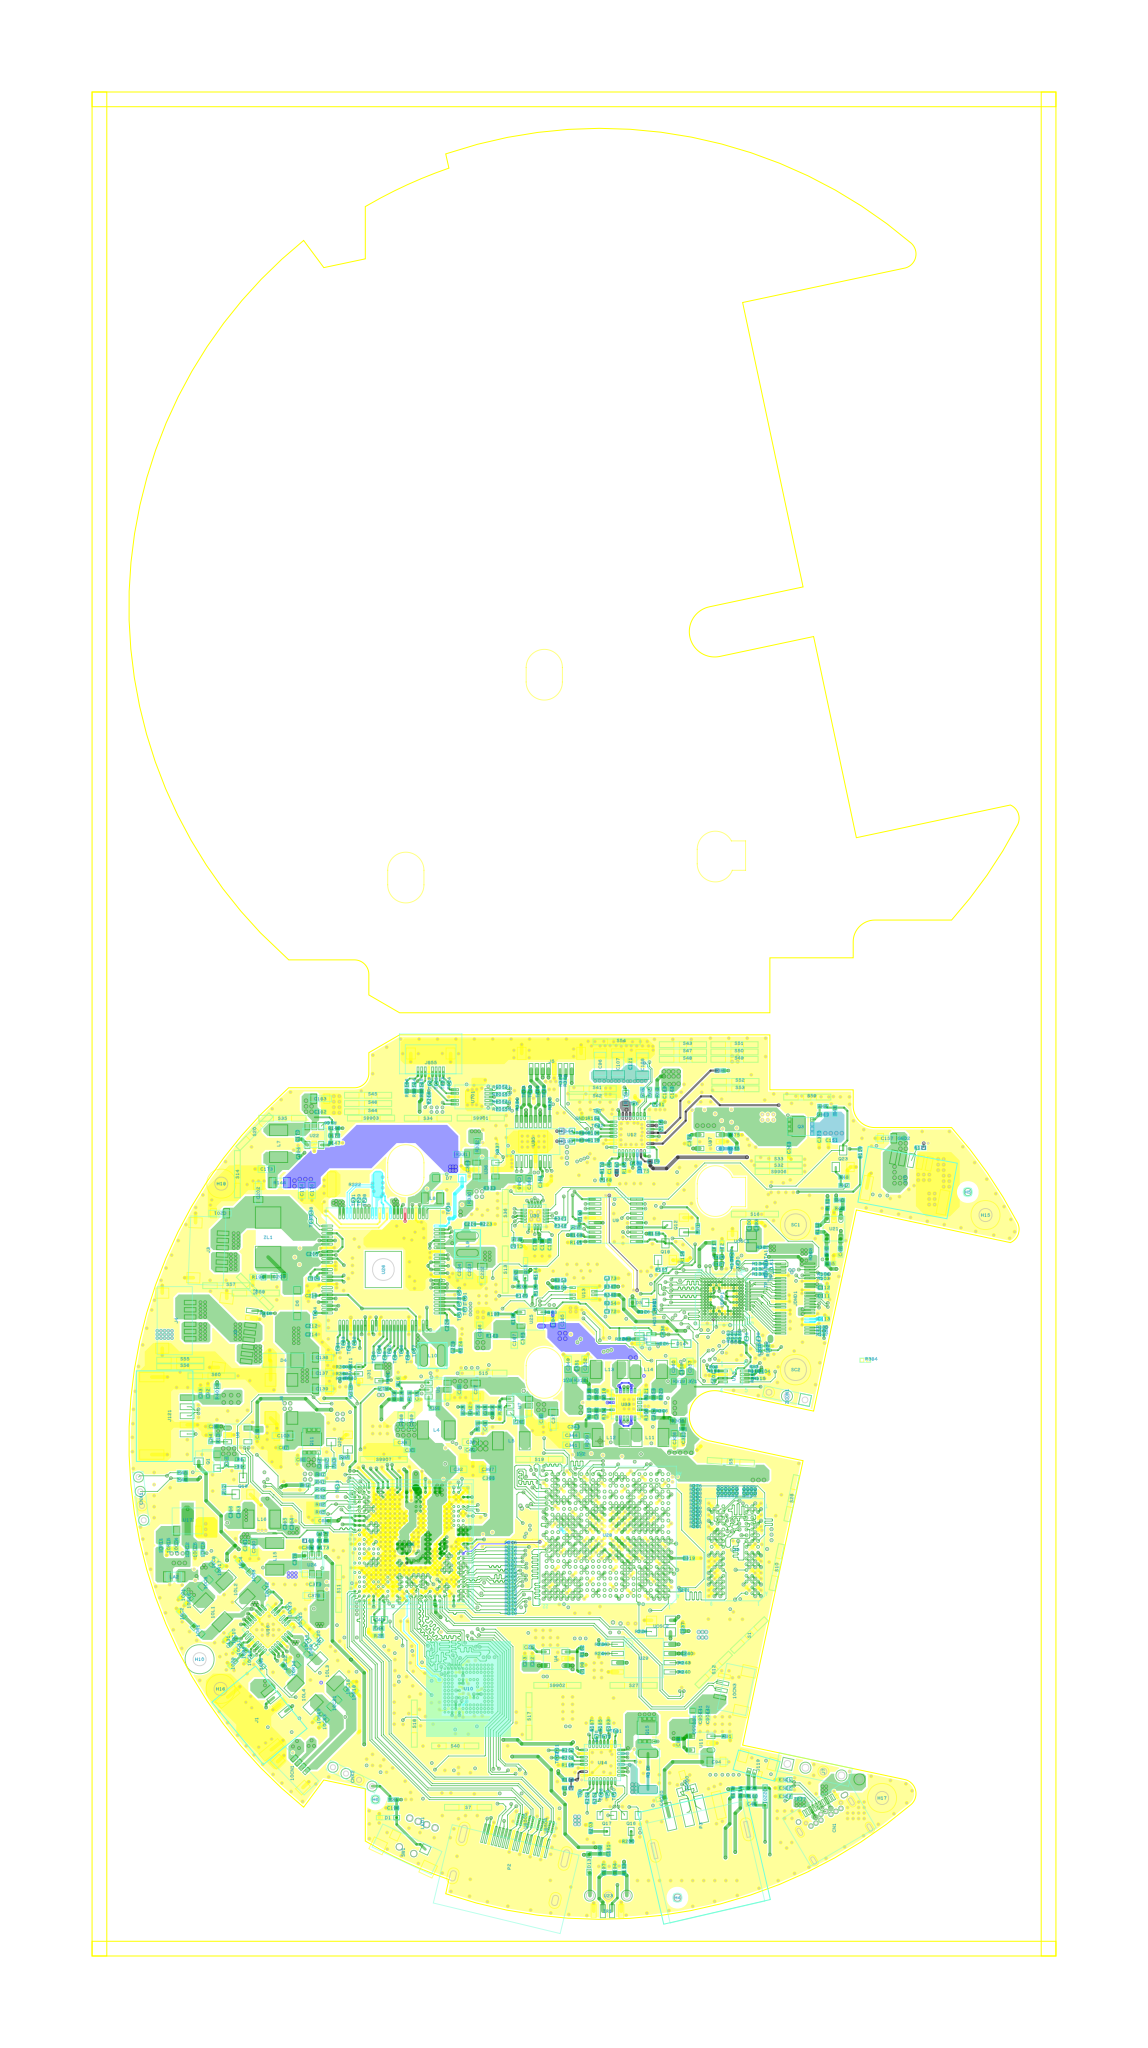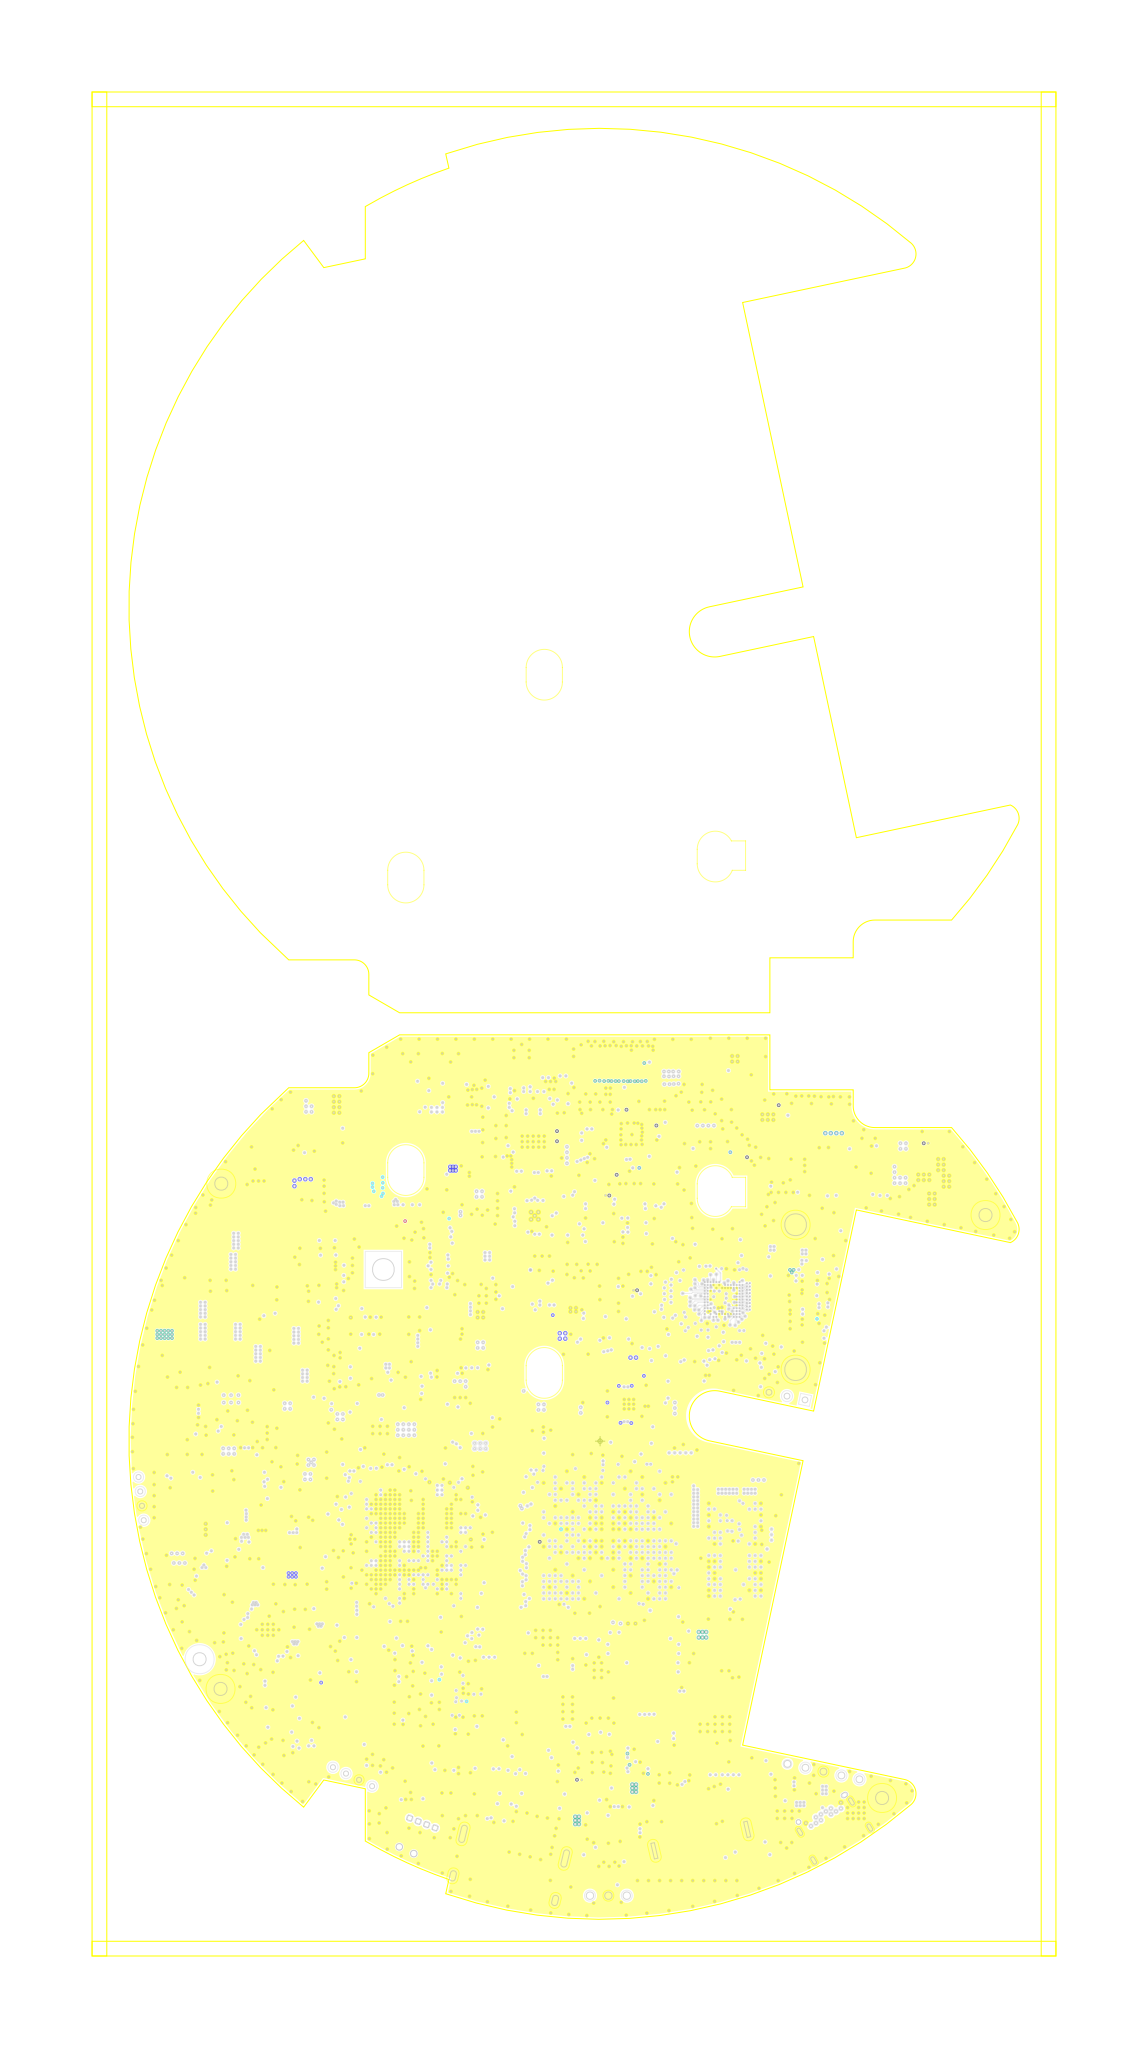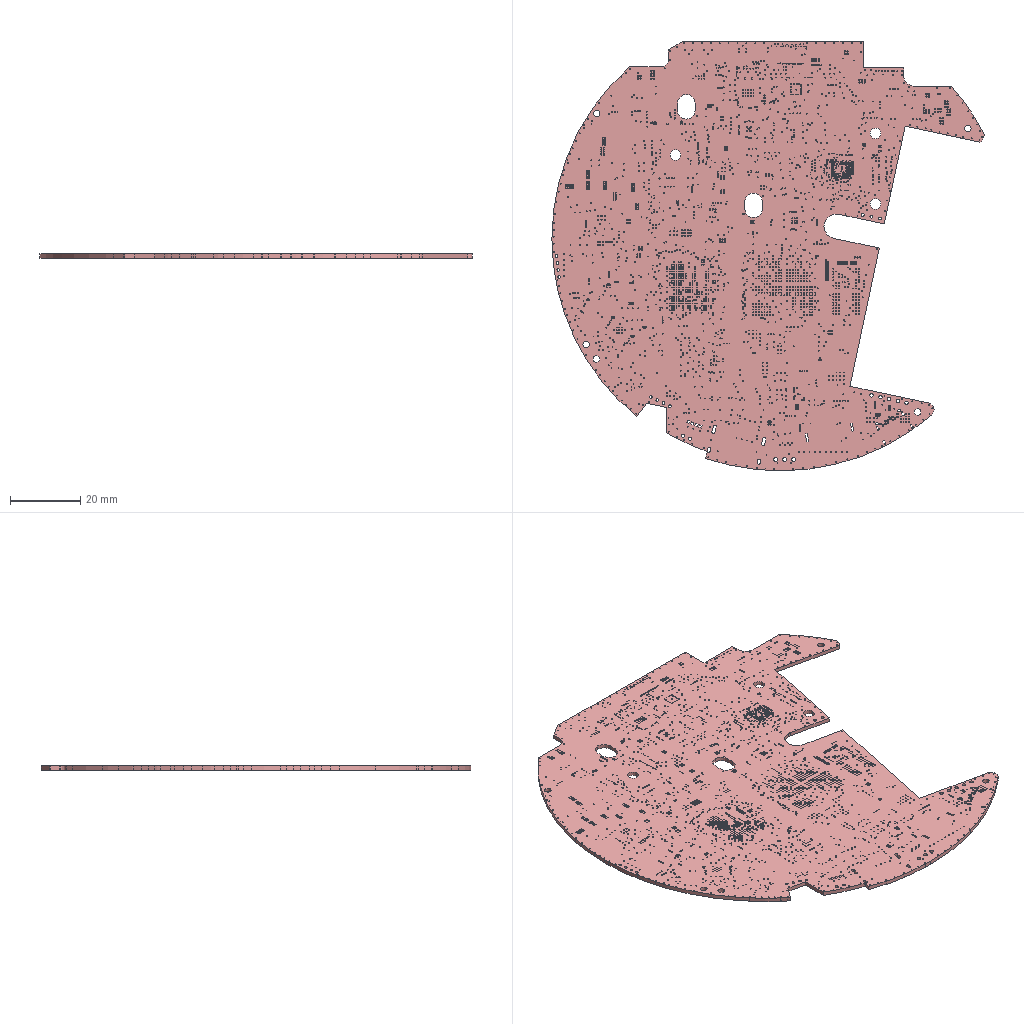Circuit board layout | Cadence Allegro | box 122.8 x 122.1 x 1.1 mm
Layer stack:
# Cadence Allegro layer stack of  (unit mm; from the constraint file cross-section; dielectric type: 0 not recorded (Allegro does not mark core vs prepreg), 3 surface material)
index,name,kind,layer,copper_thickness_mm,dielectric_type,dielectric_thickness_mm,dielectric_material,dielectric_constant
0,Top Surface,other,,,,,,
1,TOP,copper,TOP,0.0305,,,,
2,Dielectric1,dielectric,,,0,0.2032,FR-4,4.5
3,GND1,copper,GND1,0.0305,,,,
4,Dielectric2,dielectric,,,0,0.2032,FR-4,4.5
5,POWER,copper,POWER,0.0305,,,,
6,Dielectric3,dielectric,,,0,0.2032,FR-4,4.5
7,S1,copper,S1,0.0305,,,,
8,Dielectric4,dielectric,,,0,0.2032,FR-4,4.5
9,GND2,copper,GND2,0.0305,,,,
10,Dielectric5,dielectric,,,0,0.2032,FR-4,4.5
11,BOTTOM,copper,BOTTOM,0.0305,,,,
12,Bottom Surface,other,,,,,,
# drill layer pairs: low layer,high layer
drill_pair,TOP,BOTTOM
drill_pair,GND2,BOTTOM
drill_pair,TOP,GND1
drill_pair,GND1,GND2
Part placement, first 548 of 1231 lines:
REFDES,COMP_VALUE,SYM_NAME,SYM_X,SYM_Y,SYM_ROTATE,SYM_MIRROR
1C1,47uF/16V,C1206,-1850.000,-785.000,45.000,YES
1C2,47uF/16V,C1206,-1512.000,-901.000,90.000,YES
1V1,TP40,TP06MM,450.000,67.000,0.000,NO
1V2,TP40,TP06MM,-104.000,-69.000,0.000,NO
1V3,TP40,TP06MM,-177.000,331.000,0.000,NO
3V1,TP40,TP06MM,503.000,325.000,0.000,NO
10C1,0.1uF/16V,C0402,-2265.018,-836.124,45.000,NO
10C2,390pF/25V,C0402,-2272.039,-938.625,315.000,NO
10C3,470nF/16V,C0603,-2142.487,-771.091,225.000,NO
10C4,390pF/25V,C0402,-1952.426,-661.238,315.000,NO
10C5,1nF/25V,C0402,-1964.000,-908.000,135.000,YES
10C6,0.1uF/16V,C0402,-1818.000,-909.000,135.000,YES
10C7,22nF/16V,C0402,-1875.000,-951.000,45.000,YES
10C8,0.1uF/16V,C0402,-2099.454,-658.561,45.000,NO
10C9,1nF/25V,C0402,-1994.000,-1209.000,45.000,NO
10C10,0.1uF/16V,C0402,-1990.000,-1060.000,135.000,NO
10C11,100pF/25V,C0402,-1964.000,-1121.000,45.000,NO
10C12,22nF/16V,C0402,-1810.000,-807.000,135.000,NO
10C13,1uF/10V,C0402,-1685.000,-915.000,315.000,NO
10C14,22nF/16V,C0402,-1595.043,-1094.749,225.000,NO
10C15,1uF/10V,C0402,-1628.000,-972.000,315.000,NO
10C16,1uF/10V,C0402,-1904.999,-1180.000,225.000,NO
10C17,22nF/16V,C0402,-1658.000,-1144.000,180.000,YES
10C18,0.1uF/16V,C0402,-1369.271,-1335.668,225.000,NO
10C19,0.1uF/16V,C0402,-1695.000,-1021.000,270.000,YES
10C20,390pF/25V,C0402,-1530.000,-1070.000,135.000,NO
10C21,470nF/16V,C0603,-1443.518,-1424.056,225.000,NO
10C22,390pF/25V,C0402,-1710.000,-1204.999,225.000,NO
10C23,0.1uF/16V,C0402,-1496.551,-1526.586,225.000,NO
10C24,1nF/25V,C0402,-2302.000,-567.000,270.000,NO
10C25,1nF/25V,C0402,-2200.000,-591.000,270.000,NO
10CN1,4PIN-2.54-L-H-G,CN1X4-0P8MM,-1660.553,-1724.570,314.267,NO
10CN3,4PIN-2.54-L-H-G,CN1X4-1MM,739.633,-1349.018,78.167,NO
10FB1,100R/100M,L1206,-1618.000,-901.000,270.000,YES
10L1,10uH_150M-LF,MWSA0402S,-2103.597,-930.190,135.000,NO
10L2,10uH_150M-LF,MWSA0402S,-1979.853,-806.447,135.000,NO
10L3,10uH_150M-LF,MWSA0402S,-1482.409,-1250.815,315.000,NO
10L4,10uH_150M-LF,MWSA0402S,-1610.000,-1380.000,315.000,NO
10R1,3.3R,R0603,-2185.000,-1030.000,135.000,NO
10R2,4.7K,R0402,-1933.000,-881.000,135.000,YES
10R3,3.3R,R0603,-1881.716,-731.949,135.000,NO
10R4,NC,R0402,-1989.000,-981.000,225.000,YES
10R5,3.3K,R0402,-1935.000,-1150.001,225.000,NO
10R6,NC,R0402,-1840.000,-1211.000,315.000,NO
10R7,4K7,R0402,-2019.000,-951.000,45.000,YES
10R8,100R,R0402,-1642.000,-1255.000,0.000,YES
10R9,3.3R,R0603,-1571.000,-1137.000,45.000,NO
10R10,100R,R0402,-1642.000,-1214.000,0.000,YES
10R11,0R,R0402,-2386.000,-567.000,270.000,NO
10R12,4K7,R0402,-2242.000,-591.000,90.000,NO
10R13,0R,R0402,-2158.000,-591.000,270.000,NO
10R14,3.3R,R0603,-1664.999,-1235.000,45.000,NO
10R15,NC,R0402,-2344.000,-567.000,270.000,NO
10R16,4.7K,R0402,-2233.198,-867.944,225.000,NO
10R17,4.7K,R0402,-2067.635,-690.381,225.000,NO
10R18,4.7K,R0402,-1337.452,-1367.487,45.000,NO
10R19,4.7K,R0402,-1528.370,-1494.767,45.000,NO
C1,0.1uF/25V,C0402,-710.000,1518.000,0.000,YES
C2,NC/22pF,C0402,-830.000,1320.000,270.000,YES
C3,0.1uF/25V,C0402,-2123.000,-318.000,270.000,YES
C4,22pF/25V,C0402,-2286.000,-169.000,180.000,YES
C5,10uF/16V,C0805,-509.000,1426.000,270.000,YES
C6,0.1uF/25V,C0402,-586.000,1427.000,270.000,YES
C7,22uF/10V,C0603,-789.000,1730.000,180.000,YES
C8,0.1uF/25V,C0402,-802.000,1776.000,180.000,YES
C9,10uF/16V,C0805,-2219.000,-538.000,180.000,YES
C10,0.1uF/25V,C0402,-2218.000,-461.000,180.000,YES
C11,0.1uF/25V,C0402,-1869.000,-431.000,180.000,YES
C12,NC/0.1uF,C0402,-815.000,1385.000,0.000,YES
C13,22uF/6.3V,C0603,-1869.000,-386.000,180.000,YES
C14,0.47uF/16V,C0402,-2029.000,-110.000,270.000,NO
C15,33pF/25V,C0402,-1649.000,-161.000,0.000,YES
C16,10uF/6.3V,C0603,-1761.000,-169.000,180.000,YES
C17,0.1uF/25V,C0402,-1761.000,-220.000,180.000,YES
C18,22uF/6.3V,C0603,-1521.000,-240.000,180.000,YES
C19,0.1uF/25V,C0402,-1526.000,-192.000,180.000,YES
C20,0.47uF/16V,C0402,-1727.000,-450.000,0.000,YES
C21,0.01uF/25V,C0402,-387.000,-1119.000,180.000,NO
C22,2.2uF/10V,C0402,-368.000,-1197.000,90.000,NO
C23,0.1uF/25V,C0402,-409.000,-1197.000,90.000,NO
C24,0.1uF/25V,C0402,-899.000,179.000,180.000,NO
C25,22pF/25V,C0402,-1118.000,245.000,90.000,NO
C26,0.1uF/25V,C0402,-2100.000,80.000,180.000,NO
C27,10uF/16V,C0805,-676.000,280.000,270.000,NO
C28,0.1uF/25V,C0402,-765.000,280.000,270.000,NO
C29,2.2uF/10V,C0402,-1862.000,39.000,270.000,NO
C30,0.1uF/25V,C0402,-1034.000,-49.000,180.000,NO
C31,0.47uF/16V,C0402,-995.000,245.000,270.000,NO
C32,22uF/6.3V,C0603,-770.000,-153.000,0.000,NO
C33,10uF/6.3V,C0603,-1074.000,-7.000,180.000,NO
C34,47nF/10V,C0402,-2115.000,15.000,90.000,NO
C35,22pF/25V,C0402,-625.000,168.000,90.000,NO
C36,0.1uF/25V,C0402,-441.000,105.000,180.000,NO
C37,10uF/16V,C0805,-254.000,121.000,270.000,NO
C38,0.1uF/25V,C0402,-320.000,122.000,270.000,NO
C39,22uF/6.3V,C0603,-702.000,-5.000,180.000,NO
C40,0.1uF/25V,C0402,-706.000,-47.000,180.000,NO
C41,0.47uF/16V,C0402,-625.000,82.000,270.000,NO
C42,3.3nF/25V,C0402,-705.000,168.000,90.000,NO
C43,10uF/6.3V,C0603,-1199.000,-971.001,0.000,NO
C44,0.1uF/25V,C0402,-1203.000,-1017.000,0.000,NO
C45,33pF/25V,C0402,-934.000,-1060.000,0.000,YES
C46,33pF/25V,C0402,823.000,-1972.000,180.000,NO
C47,33pF/25V,C0402,-938.000,-838.000,180.000,YES
C48,NC/1000pF,C0402,-1342.000,-113.000,180.000,YES
C49,0.1uf/0402/10%/X7R,C0402,1305.000,1030.000,90.000,NO
C50,22uF/6.3V,C0603,-893.000,-464.000,180.000,YES
C51,0.1uF/25V,C0402,-1012.000,-673.000,90.000,YES
C52,10uF/6.3V,C0603,-1114.000,-559.000,0.000,YES
C53,10uF/6.3V,C0603,-944.000,-266.000,0.000,YES
C54,0.1uF/25V,C0402,-912.000,-574.000,180.000,YES
C55,NC/22uF/6.3V,C0603,-753.000,-433.000,0.000,YES
C56,10uF/6.3V,C0603,-662.000,-501.000,90.000,YES
C57,0.1uF/25V,C0402,-820.000,-599.000,180.000,YES
C58,10uF/6.3V,C0603,-781.000,-979.000,180.000,YES
C59,10uF/6.3V,C0603,-1089.000,-610.000,0.000,YES
C60,0.1uF/25V,C0402,-1021.000,-512.000,180.000,YES
C61,0.1uF/25V,C0402,-1018.000,-553.000,180.000,YES
C62,10uF/6.3V,C0603,-659.000,-282.000,270.000,YES
C63,10uF/6.3V,C0603,-1303.000,-448.000,90.000,YES
C64,10uF/6.3V,C0603,-1358.000,-432.000,90.000,YES
C65,4.7uF/16V,C0603,-1178.000,-937.000,90.000,YES
C66,4.7uF/16V,C0603,-826.000,-885.000,270.000,YES
C67,10uF/6.3V,C0603,-1448.000,-539.000,90.000,YES
C68,4.7uF/16V,C0603,-1505.000,-432.000,180.000,NO
C69,4.7uF/16V,C0603,-1395.000,-539.000,90.000,YES
C70,0.1uF/25V,C0402,-863.000,-1001.000,90.000,YES
C71,0.1uF/25V,C0402,-840.000,-75.000,270.000,YES
C72,0.47uF/16V,C0402,-1114.000,-89.000,90.000,YES
C73,2.2uF/10V,C0402,-612.000,-516.000,270.201,YES
C74,0.47uF/16V,C0402,-1155.000,-88.000,270.000,YES
C75,0.47uF/16V,C0402,-1131.000,-25.000,0.000,YES
C76,2.2uF/10V,C0402,-1279.000,-88.000,270.000,YES
C77,1uF/10V,C0402,-800.000,-75.000,270.000,YES
C78,0.1uF/25V,C0402,-1217.000,-109.000,180.000,YES
C79,1nF/25V,C0402,-1217.000,-199.000,90.000,YES
C80,0.1uF/25V,C0402,-1175.000,-199.000,90.000,YES
C81,0.1uF/25V,C0402,-828.000,-1419.000,0.000,YES
C82,2.2uF/10V,C0402,-729.000,-1535.000,180.000,YES
C83,2.2uF/10V,C0402,-695.000,-1344.000,0.000,YES
C84,0.1uF/25V,C0402,-695.000,-1289.000,180.000,YES
C85,0.1uf/0402/10%/X7R,C0402,1250.000,965.000,0.000,NO
C86,0.1uF/25V,C0402,-1525.000,-120.000,90.000,NO
C87,0.1uF/25V,C0402,-1720.000,-35.000,180.000,NO
C88,0.1uF/25V,C0402,-1625.000,-100.000,180.000,NO
C89,0.1uF/25V,C0402,-526.000,-1932.000,90.000,YES
C90,1uF/10V,C0402,-481.000,-2192.000,90.000,YES
C91,1uF/10V,C0402,424.000,-1634.000,90.000,NO
C92,2.2uF/10V,C0402,-2130.000,260.000,90.000,NO
C93,0.1uF/25V,C0402,-2170.000,260.000,90.000,NO
C94,22uF/16V,C0805,632.000,-1743.000,180.000,NO
C95,22uF-25V,C1206,260.000,-1615.000,89.931,YES
C96,22uF-25V,C1206,0.000,2050.000,90.000,NO
C97,1uF,C0402,95.000,-1644.000,359.931,YES
C98,1uF,C0402,60.000,-1570.000,0.069,YES
C99,2.2NF,C0402,200.000,-1805.000,180.069,YES
C100,0.1uF,C0201,809.000,1173.000,90.000,NO
C101,0.1uF,C0201,616.000,343.000,90.000,NO
C102,2.2NF,C0402,95.000,-1765.000,0.000,YES
C103,22uF/16V,C0805,-1720.000,30.000,180.000,NO
C104,0.1uF,C0201,891.000,380.000,0.000,NO
C105,0.1uF,C0201,923.000,959.000,90.000,YES
C106,0.1uF,C0201,485.000,1125.000,270.000,YES
C107,22uF-25V,C1206,97.000,2050.000,90.000,NO
C108,22uF-25V,C1206,230.000,2047.000,90.000,NO
C109,0.22uF,C0402,550.000,761.000,89.931,YES
C110,0.1uF,C0201,499.000,715.000,179.931,YES
C111,0.1uF,C0402,1215.000,790.000,0.000,NO
C112,0.1uF,C0402,1215.000,835.000,0.000,NO
C113,0.1uF,C0402,1215.000,665.000,0.000,NO
C114,0.1uF,C0201,1065.000,997.000,270.000,YES
C115,0.1uF,C0201,626.000,833.000,270.000,YES
C116,0.1uF,C0201,662.000,833.000,270.000,YES
C117,0.1uF,C0201,711.000,896.000,270.000,YES
C118,0.1uF,C0201,639.000,747.000,180.000,YES
C119,0.1uF,C0201,684.000,669.000,90.000,YES
C120,0.1uF,C0201,762.000,895.000,270.000,YES
C121,100nF,C0402,164.000,2051.000,90.000,NO
C122,0.1uF,C0201,673.000,896.000,270.000,YES
C123,0.1uF,C0201,699.000,833.000,270.000,YES
C124,0.1uF,C0201,736.000,833.000,270.000,YES
C125,0.1uF,C0201,748.000,692.000,270.000,YES
C126,1uF,C0402,787.000,694.000,270.000,YES
C127,0.1uF,C0201,645.000,963.000,0.000,NO
C128,10nF,C0201,645.000,1001.000,180.000,NO
C129,0.1uF,C0201,589.000,833.000,270.000,YES
C130,0.1uF,C0201,642.000,590.000,0.000,YES
C131,0.1uF/25V,C0402,-2020.000,-1090.000,135.000,NO
C132,1uF/10V,C0402,-2070.000,-680.000,0.000,YES
C133,0.1uF/25V,C0402,-2070.000,-760.000,0.000,YES
C134,0.1uF/25V,C0402,-2320.000,-745.000,180.000,YES
C135,0.1uF/25V,C0402,-2085.000,-585.000,90.000,YES
C136,0.1uF/25V,C0402,-1920.000,-615.000,0.000,YES
C137,22uF/16V,C0805,-1511.000,370.000,0.000,NO
C138,22uF/16V,C0805,-1510.000,455.000,0.000,NO
C139,22uF/16V,C0805,-1510.000,285.000,0.000,NO
C140,0.1uF,C0201,696.000,504.000,0.000,YES
C141,0.1uF,C0201,802.000,528.000,180.000,YES
C142,0.1uF,C0201,799.000,895.000,270.000,YES
C143,0.1uF,C0201,647.000,687.000,270.000,YES
C144,0.1uF,C0201,639.000,784.000,180.000,YES
C145,0.1uF,C0201,499.000,753.000,180.000,YES
C146,0.1uF,C0201,752.000,769.000,180.000,YES
C147,0.1uF,C0201,1035.000,997.000,270.000,YES
C148,10nF,C0402,390.000,1895.000,270.000,NO
C149,1nF,C0402,350.000,1895.000,270.000,NO
C150,22uF-25V,C1206,150.000,1900.000,0.000,YES
C151,100nF,C0402,1258.000,1636.000,180.000,NO
C152,22uF-25V,C1206,1095.000,1775.000,270.000,YES
C153,22uF-25V,C1206,1200.000,1775.000,270.000,YES
C154,22uF-25V,C1206,1305.000,1775.000,270.000,YES
C155,NC,C0402,786.000,2082.000,0.000,YES
C156,NC,C0402,885.000,1500.000,0.000,YES
C157,10uF-25V,C0805,1559.000,1646.000,180.000,NO
C158,47nF,C0402,330.000,1715.000,270.000,NO
C159,47nF,C0402,290.000,1520.000,0.000,NO
C160,100nF,C0402,1540.000,1440.000,0.000,YES
C161,470nF,C0402,316.000,1830.000,180.000,NO
C162,0.1uF/16V,C0402,-1247.000,-936.000,180.000,YES
C163,1nF,C0402,195.000,1510.000,180.000,NO
C164,1uF,C0402,140.000,1760.000,270.000,YES
C165,220pF,C0402,50.000,1485.000,90.000,NO
C166,1nF,C0402,-55.000,1605.000,270.000,YES
C167,2.2uF,C0402,260.000,1655.000,180.000,YES
C168,1nF,C0402,30.000,1420.000,180.000,NO
C169,10pF,C0402,65.000,1615.000,90.000,YES
C170,0.1uF,C0402,-1643.000,1659.000,270.000,NO
C171,NC,C0402,-107.000,-1864.000,0.000,YES
C172,220pF,C0402,-1444.000,1661.000,180.000,NO
C173,22uF,C0603,-1811.000,1479.000,180.000,NO
C174,22uF,C0603,-1620.000,1365.000,270.000,NO
C175,1uF,C0402,233.000,1468.000,0.000,NO
C176,10uF,C0603,-1565.000,1365.000,90.000,NO
C177,0.1uF/25V,C0402,-315.000,1070.000,270.000,NO
C178,0.1uF/25V,C0402,-275.000,1070.000,270.000,NO
C179,0.1uF/25V,C0402,-355.000,1070.000,270.000,NO
C180,0.1uF/25V,C0402,-454.000,1059.000,0.000,NO
C181,33pF/25V,C0402,45.000,-2225.000,90.000,NO
C182,0.1uF,C0402,-1520.000,1790.000,0.000,NO
C183,10uF,C0805,-1520.000,1861.000,180.000,NO
C184,0.1uF,C0201,-256.000,647.000,90.000,NO
C185,10uF,C0603,-206.000,656.000,90.000,NO
C186,22uF,C0603,-654.000,601.000,90.000,NO
C187,22uF,C0603,-466.000,550.000,270.000,NO
C188,10uF,C0603,-905.000,1260.000,0.000,YES
C189,10uF,C0805,-1005.000,1200.000,90.000,YES
C190,22uF,C0805,-1370.000,1055.000,180.000,YES
C191,22uF,C0805,-1370.000,1135.000,180.000,YES
C192,1uF,C0402,60.000,-1930.000,270.000,YES
C193,1uF,C0402,45.000,-1545.000,90.000,NO
C194,2.2uF/10V,C0402,80.000,-2328.000,90.000,NO
C195,0.47uF/16V,C0402,344.000,1503.000,0.000,YES
C196,0.1uF/25V,C0402,-1123.000,-1993.000,180.000,NO
C197,0.1uF/25V,C0402,20.000,-2328.000,90.000,NO
C198,100NF,C0402,-98.217,-1234.055,90.000,NO
C199,1uF,C0402,-970.000,1315.000,180.000,YES
C200,0.1uF,C0402,-1564.000,1017.000,180.000,NO
C201,22uF,C0805,-2064.000,1239.000,180.000,NO
C202,22uF,C0805,-1857.000,1349.000,90.000,NO
C203,1.2nF,C0603,-1743.000,894.000,180.000,NO
C204,10pF,C0402,-1555.000,884.000,180.000,NO
C205,1uF,C0603,-905.000,1205.000,0.000,YES
C206,1uF,C0603,-905.000,1155.000,0.000,YES
C207,22uF,C0805,-1595.000,1000.000,0.000,YES
C208,22uF,C0805,-1595.000,1085.000,0.000,YES
C209,1uF,C0603,-905.000,1105.000,0.000,YES
C210,0.1uF,C0201,-1568.000,791.000,180.000,NO
C211,1uF,C0402,-970.000,870.000,0.000,YES
C212,1uF,C0402,-1568.639,626.410,0.000,NO
C213,1uF,C0402,-1065.000,1145.000,90.000,YES
C214,1uF,C0402,-1569.000,580.000,0.000,NO
C215,2.2uF,C0402,-870.000,985.000,180.000,YES
C216,4.7uF,C0402,-870.000,1025.000,180.000,YES
C217,1uF,C0402,-809.000,863.000,180.000,YES
C218,0.1uF,C0402,-783.000,1094.000,90.000,YES
C219,10uF,C0805,-1000.000,1010.000,0.000,YES
C220,10uF,C0805,-1000.000,930.000,0.000,YES
C221,470pF,C0402,-705.000,1180.000,180.000,NO
C222,47uF,C0805,-640.000,915.000,270.000,NO
C223,22uF,C0603,-710.000,930.000,270.000,NO
C224,22uF,C0603,-765.000,930.000,270.000,NO
C225,0.1uF,C0402,-832.000,630.000,270.000,NO
C226,10uF,C0805,-999.000,767.000,0.000,YES
C227,10uF,C0805,-855.000,780.000,180.000,YES
C228,470pF,C0402,-800.000,510.000,90.000,NO
C229,47uF,C0805,-876.000,564.000,270.000,YES
C230,22uF,C0603,-1055.000,540.000,0.000,YES
C231,22uF,C0603,-954.000,561.000,270.000,YES
C232,1uF,C0402,-1005.000,1075.000,0.000,YES
C233,1uF,C0402,-870.000,905.000,0.000,YES
C234,1uF,C0402,-970.000,830.000,0.000,YES
C235,1uF,C0402,-870.000,945.000,0.000,YES
C236,0.1uF,C0201,340.000,595.000,270.000,NO
C237,0.1uF,C0201,449.000,-1017.000,90.000,NO
C238,0.1uF,C0201,70.000,-944.000,270.000,YES
C239,0.1uF,C0201,192.000,-945.000,90.000,YES
C240,0.1uF,C0201,472.000,-1154.000,0.000,NO
C241,NC/13pF,C0402,-227.000,-504.000,180.000,YES
C242,10nF,C0201,874.000,-386.000,90.000,YES
C243,10nF,C0201,874.000,-668.000,270.000,YES
C244,10nF,C0201,606.000,-847.000,0.000,YES
C245,10nF,C0201,859.000,-811.000,180.000,YES
C246,10nF,C0201,638.000,-653.000,0.000,YES
C247,0.1uF,C0201,606.000,-712.000,180.000,YES
C248,10nF,C0201,859.000,-746.000,180.000,YES
C249,10nF,C0201,842.000,-542.000,90.000,YES
C250,10nF,C0201,874.000,-448.000,90.000,YES
C251,10nF,C0201,590.000,-415.000,270.000,YES
C252,10nF,C0201,590.000,-354.000,270.000,YES
C253,0.1uF,C0201,590.000,-638.000,90.000,YES
C254,0.1uF,C0201,182.000,-415.000,0.000,YES
C255,10nF,C0201,213.000,-671.000,180.000,YES
C256,0.1uF,C0201,861.000,-618.000,180.000,YES
C257,0.1uF,C0201,213.000,-634.000,180.000,YES
C258,10nF,C0201,923.000,-618.000,180.000,YES
C259,0.1uF,C0201,618.000,-480.000,270.000,YES
C260,10nF,C0201,893.000,-502.000,0.000,YES
C261,0.1uF,C0201,581.000,-480.000,270.000,YES
C262,10nF,C0201,893.000,-540.000,0.000,YES
C263,0.1uF,C0201,954.000,-443.000,270.000,YES
C264,0.47uF,C0201,293.000,-243.000,270.000,YES
C265,4.7uF,C0402,293.000,-323.000,180.000,YES
C266,0.47uF,C0201,324.000,-180.000,90.000,YES
C267,4.7uF,C0402,-22.000,-691.000,0.000,YES
C268,47uF,C0805,389.000,-130.000,90.000,YES
C269,47uF,C0805,472.000,-130.000,90.000,YES
C270,4.7uF,C0402,40.000,-688.000,90.000,YES
C271,4.7uF,C0402,42.000,-576.000,270.000,YES
C272,0.47uF,C0201,164.000,-652.000,270.000,YES
C273,0.47uF,C0201,164.000,-590.000,270.000,YES
C274,0.47uF,C0201,151.000,-541.000,0.000,YES
C275,0.47uF,C0201,103.000,-588.000,270.000,YES
C276,0.47uF,C0201,-7.000,-415.000,180.000,YES
C277,0.47uF,C0201,-39.000,-569.000,0.000,YES
C278,0.47uF,C0201,-39.000,-606.000,180.000,YES
C279,4.7uF,C0402,-53.000,-464.000,90.000,YES
C280,47uF,C0805,637.000,-130.000,90.000,YES
C281,47uF,C0805,-22.000,-975.000,0.000,YES
C282,47uF,C0805,-83.000,30.000,0.000,YES
C283,4.7uF,C0402,83.000,-511.000,0.000,YES
C284,0.47uF,C0201,86.000,-382.000,0.000,YES
C285,0.47uF,C0201,103.000,-460.000,90.000,YES
C286,0.47uF,C0201,133.000,-369.000,90.000,YES
C287,4.7uF,C0402,43.000,-446.000,90.000,YES
C288,47uF,C0805,-83.000,111.000,0.000,YES
C289,47uF,C0805,-227.000,-81.000,270.000,YES
C290,4.7uF,C0402,-181.000,-365.000,90.000,YES
C291,4.7uF,C0402,-39.000,-193.000,0.000,YES
C292,0.47uF,C0201,-182.000,-294.000,270.000,YES
C293,0.47uF,C0201,-258.000,-195.000,0.000,YES
C294,0.47uF,C0201,198.000,-337.000,270.000,YES
C295,0.47uF,C0201,247.000,-792.000,180.000,YES
C296,22uF,C0603,-75.000,-105.000,270.000,YES
C297,22uF,C0603,-20.000,-105.000,270.000,YES
C298,22uF,C0603,222.000,-124.000,270.000,YES
C299,47uF,C0805,-144.000,-81.000,270.000,YES
C300,4.7uF,C0402,53.000,-319.000,0.000,YES
C301,4.7uF,C0402,-22.000,-881.000,90.000,YES
C302,0.47uF,C0201,-22.000,-810.000,270.000,YES
C303,0.47uF,C0201,-11.000,-730.000,0.000,YES
C304,0.47uF,C0201,-133.000,-225.000,180.000,YES
C305,0.47uF,C0201,103.000,-210.000,90.000,YES
C306,0.47uF,C0201,85.000,-636.000,0.000,YES
C307,10uF,C0603,102.000,-703.000,90.000,YES
C308,47uF,C0805,-320.000,-309.000,270.000,YES
C309,4.7uF,C0402,-86.000,-371.000,90.000,YES
C310,4.7uF,C0402,-216.000,-395.000,270.000,YES
C311,0.47uF,C0201,-292.000,-384.000,180.000,YES
C312,0.47uF,C0201,-103.000,-447.000,180.000,YES
C313,0.47uF,C0201,-125.000,-364.000,90.000,YES
C314,0.47uF,C0201,-164.000,-574.000,0.000,YES
C315,0.47uF,C0201,276.000,-697.000,180.000,YES
C316,0.47uF,C0201,340.000,-507.000,180.000,YES
C317,0.47uF,C0201,339.000,-386.000,0.000,YES
C318,0.47uF,C0201,370.000,-289.000,0.000,YES
C319,4.7uF,C0402,482.000,-635.984,0.000,NO
C320,47uF,C0805,936.000,-327.000,270.000,YES
C321,0.1uF,C0201,200.000,140.000,90.000,YES
C322,22uF,C0603,-25.000,262.000,180.000,YES
C323,22uF,C0603,407.000,17.000,0.000,YES
C324,220pF,C0402,290.000,145.000,270.000,NO
C325,0.1uF,C0201,452.000,19.000,90.000,NO
C326,22uF,C0603,404.000,16.000,90.000,NO
C327,47uF,C0805,-137.000,-1004.000,270.000,YES
C328,4.7uF,C0402,-294.000,-699.000,180.000,YES
C329,4.7uF,C0402,-240.000,-658.000,180.000,YES
C330,0.47uF,C0201,-103.000,-793.000,180.000,YES
C331,0.47uF,C0201,-243.000,-872.000,90.000,YES
C332,0.47uF,C0201,-86.000,-683.000,270.000,YES
C333,0.47uF,C0201,-166.000,-667.000,180.000,YES
C334,0.1uF,C0201,80.000,140.000,90.000,YES
C335,22uF,C0603,200.000,45.000,270.000,YES
C336,0.47uF,C0201,164.000,-464.000,90.000,YES
C337,4.7uF,C0402,1.000,-511.000,180.000,YES
C338,47uF,C0805,555.000,-130.000,90.000,YES
C339,0.1uF,C0201,80.000,210.000,0.000,YES
C340,22uF,C0603,-25.000,210.000,180.000,YES
C341,22uF,C0603,-156.000,-22.000,0.000,NO
C342,220pF,C0402,-20.000,150.000,270.000,NO
C343,0.1uF,C0201,-143.000,78.000,0.000,NO
C344,22uF,C0603,-156.000,32.000,0.000,NO
C345,0.1uF,C0201,200.000,260.000,270.000,YES
C346,22uF,C0603,250.000,245.000,270.000,YES
C347,0.1uF,C0201,80.000,260.000,270.000,YES
C348,22uF,C0603,10.000,316.000,180.000,YES
C349,22uF,C0603,-174.000,417.000,270.000,NO
C350,220pF,C0402,-20.000,255.000,90.000,NO
C351,0.1uF,C0201,-127.000,410.000,270.000,NO
C352,22uF,C0603,-81.000,417.000,270.000,NO
C353,NC/10nF,C0201,160.000,140.000,90.000,YES
C354,NC/10nF,C0201,120.000,260.000,270.000,YES
C355,NC/10nF,C0201,120.000,140.000,90.000,YES
C356,NC/10nF,C0201,160.000,260.000,270.000,YES
C357,22uF,C0603,488.000,405.000,270.000,NO
C358,220pF,C0402,290.000,255.000,90.000,NO
C359,0.1uF,C0201,443.000,390.000,270.000,NO
C360,22uF,C0603,398.000,405.000,270.000,NO
C361,0.1uF,C0201,-232.000,1819.000,270.000,YES
C362,0.1uF,C0201,-195.000,1819.000,270.000,YES
C363,10uF,C0603,-385.000,1401.000,270.000,NO
C364,2.2uF,C0402,-325.000,1410.000,90.000,NO
C365,10uF,C0603,-439.000,1401.000,270.000,NO
C366,0.1uF,C0201,-720.000,1495.000,90.000,NO
C367,0.1uF/25V,C0402,-330.000,1165.000,180.000,YES
C368,0.1uF/25V,C0402,1025.000,1595.000,270.000,NO
C369,0.1uF/25V,C0402,1210.000,1775.000,180.000,NO
C370,0.1uF/25V,C0402,1190.000,1655.000,270.000,NO
C371,1uF/25V,C0402,95.000,-1685.000,180.000,YES
C372,1uF/10V,C0402,55.000,705.000,0.000,NO
C373,1uF/10V,C0402,55.000,885.000,0.000,NO
C374,0.01uF/25V,C0402,485.000,1635.000,270.000,NO
C375,100NF,C0402,725.000,1665.000,0.000,NO
C376,0.1uF/25V,C0402,-1659.000,-642.000,90.000,NO
C377,NC/22pF,C0402,-1507.000,-504.000,180.000,NO
C378,10uF/16V,C0805,-1553.000,-839.000,180.000,NO
C379,0.1uF/25V,C0402,-1547.000,-778.000,180.000,NO
C380,22uF/10V,C0603,-1881.000,-575.000,270.000,NO
C381,0.1uF/25V,C0402,-1928.000,-565.000,270.000,NO
C382,NC/0.1uF,C0402,-1586.000,-578.000,180.000,NO
C383,0.1uF/25V,C0402,-1963.932,-385.690,90.000,NO
C384,2.2uF/10V,C0402,-1674.999,-451.000,90.000,NO
C385,0.1uF/25V,C0402,-1712.000,-450.000,90.000,NO
C386,2.2uF/10V,C0402,-2006.518,-385.690,90.000,NO
C387,0.47uF/16V,C0402,-1368.000,-1367.000,270.000,YES
C388,22uF/6.3V,C0603,-1080.000,113.000,90.000,NO
C389,22uF/6.3V,C0603,-1024.000,112.000,90.000,NO
C390,0.1uF/25V,C0402,-835.000,-178.000,180.000,YES
C391,22uF/6.3V,C0603,-582.000,17.000,270.000,YES
C392,0.1uF/25V,C0402,-669.000,40.000,270.000,YES
C393,2.2uF,C0201,849.000,1173.000,90.000,NO
C394,0.1uF,C0402,-1639.000,1564.000,90.000,NO
C395,0.1uF,C0402,-420.000,558.000,270.000,NO
C396,0.1uF/25V,C0402,-605.000,-201.000,180.000,NO
C397,22uF/6.3V,C0603,-609.000,-153.000,180.000,NO
C4000,0.1uF/16V,C0402,-811.000,-1535.000,180.000,YES
C4001,0.1uF/16V,C0402,-745.000,-1458.000,180.000,YES
C4002,0.1uF/16V,C0402,-695.000,-1247.000,180.000,YES
C4003,0.1uF/16V,C0402,-828.000,-1458.000,0.000,YES
C4004,2.2uF/10V,C0402,-776.000,-1295.000,90.000,YES
C4005,0.1uF/16V,C0402,-683.000,-1424.000,90.000,YES
C4006,0.1uF/16V,C0402,-640.000,-1424.000,90.000,YES
C4007,2.2uF/10V,C0402,-610.000,-1341.000,270.000,YES
C4008,2.2uF/10V,C0402,-904.000,-1266.000,0.000,YES
C4017,2.2uF/10V,C0402,-1772.000,198.000,180.000,YES
C4018,0.1uF/25V,C0402,-1790.000,114.000,90.000,YES
C4019,0.1uF/25V,C0402,-1772.000,248.000,180.000,YES
C4020,0.1uF/25V,C0402,333.000,-1941.000,195.943,NO
C90441,0.1uF/25V,C0402,544.000,-1486.000,270.000,NO
C90442,2.2uF/10V,C0402,584.000,-1486.000,270.000,NO
C90446,2.2uF/10V,C0402,-625.000,1895.000,0.000,YES
C90447,0.1uF/25V,C0402,-625.000,1845.000,0.000,YES
CN1,USB Type-C Receptacle,USB_TYPE_C,1077.533,-2069.709,30.422,NO
CNX1,CON4-2.0-NC,DIP4PIN-2P0MM,-2506.759,-195.053,96.873,NO
CNX2,CON4-2.0-NC,DIP4PIN-2P0MM,-1238.203,-1874.925,334.184,NO
D1,3.3V,SOD323,-1154.500,-2046.000,0.000,NO
D2,AZC199,SOT-23-6L,-520.001,-2062.000,180.000,YES
D3,B5819W,SOD123,-1645.000,-1375.000,0.000,YES
D4,0.4KP15A,DO_214AC,-1719.000,440.000,180.000,NO
D5,RED-NC,SMD-LED,210.990,753.359,0.000,NO
D6,1N5819HW-7,SOD123,-1645.000,750.000,90.000,NO
D7,MBR0540,SOD123,-820.000,1430.000,0.000,NO
D8,ESDA18-1K,SOD523,-1105.000,1221.624,270.000,YES
D9,ESDA18-1K,SOD523,-1255.000,1220.000,270.000,YES
D10,ESDA18-1K,SOD523,-1433.376,1250.000,180.000,YES
D11,B5819W,SOD323,157.500,1250.000,180.000,YES
D12,B5819W,SOD323,162.500,1310.000,0.000,YES
D13,B5819W,SOD323,-60.000,-2292.500,270.000,NO
D14,RED-NC,SMD-LED,440.000,530.000,180.000,NO
D15,3.3V,SOD323,-405.000,937.500,270.000,NO
D16,B5819W,SOD323,133.000,1404.500,270.000,YES
D17,B5819W,SOD323,193.000,1404.500,270.000,YES
D18,NC,SOD323,-1403.000,-1503.500,90.000,YES
D2201,B5819W,SOD323,896.000,-1933.500,90.000,NO
ESD1,ESD5341N,ESD0402,1005.000,-1840.000,180.000,NO
ESD2,ESD5341N,ESD0402,1005.000,-1885.000,180.000,NO
ESD3,ESD5341N,ESD0402,1005.000,-1930.000,180.000,NO
ESD4,ESD5341N,ESD0402,1012.000,-2156.000,90.000,YES
ESD5,ESD5341N,ESD0402,-1589.000,-1487.000,270.000,YES
ESD6,ESD5341N,ESD0402,-1792.000,-1295.000,90.000,YES
ESD7,ESD5341N,ESD0402,-1866.000,-1419.000,180.000,YES
F1,BLM15PD800SN1D,R0402,619.000,1060.000,90.000,NO
F2,BLM15PD800SN1D,R0402,662.000,1060.000,90.000,NO
F3,BLM15PD800SN1D,R0402,134.000,-615.000,270.000,YES
GND1,DEO,TP06MM,-100.000,1755.000,180.000,NO
GND2,DEO,TP06MM,1650.000,1646.000,180.000,NO
H4,NC,TPAD,420.000,-2481.000,0.000,NO
H5,NC,TPAD,1997.000,1354.000,0.000,NO
H6,NC,TPAD,-1220.000,-1947.000,0.000,NO
H7,NC,TPAD,420.000,-2481.000,0.000,YES
H8,NC,TPAD,1997.000,1354.000,0.000,YES
H9,NC,TPAD,-1220.000,-1947.000,0.000,YES
H10,NC,HOLE_D1D8MM,-2175.000,-1185.000,0.000,NO
H15,NC,HOLE_D1D8MM,2093.260,1228.950,0.000,NO
H16,NC,HOLE_D1D8MM,-2061.258,-1346.315,0.000,NO
H17,NC,HOLE_D1D8MM,1531.475,-1939.054,0.000,NO
H18,NC,HOLE_D1D8MM,-2057.341,1399.627,0.000,NO
HOST_IRQ1,TP40,TP06MM,295.000,703.000,270.000,NO
IR1,AO-R123C6E,AO-R123C6E-HS,40.000,-2554.409,0.000,NO
J1,CON4,CN1X4-1P25MM-WF,-1756.142,-1411.984,309.503,NO
J2,ZYA1001-FRS08,ZYA1001-FRS08,-1922.228,434.070,83.117,NO
J3,ZYA1001-FRS06,ZYA1001-FRS06,-2055.187,933.202,87.749,NO
J4,ZYA1001-FRS06,ZYA1001-FRS06,-2226.250,556.415,90.000,NO
J5,FPC-0.5MM-SMT-08P,50208_0_8MM_8P,-170.000,2022.500,180.000,NO
J6,TLDCM7035-2-501TF,TLDCM7035,-1730.618,229.647,90.000,NO
J7,NC,SIP5P,1212.933,-1795.630,347.886,NO
J10,CON5,CN1X5-1P25MM-WF,1690.495,1525.331,349.410,NO
J119,CON3,CN1X3-0P8MM,867.231,-1814.808,164.419,NO
J121,CON7,CN1X5-1P25MM-WF,-2242.953,137.969,270.000,NO
J855,AYF530835,AYF530835,-920.000,2008.544,180.000,NO
JDMD1,AXK850145WG,AXK850145WG,1060.000,775.000,90.000,NO
L1,ATNR6045M100MT/2A,MWSA0402S,-755.000,1619.000,180.000,YES
L2,ATNR6045M6R8MT/2A,MWSA0402S,-1959.000,-276.000,0.000,YES
L3,ATNR30102R2MT,SMD03X03,-1594.000,-346.000,0.000,YES
L4,ATNR6045M2R2MT/3A,MWSA0402S,-889.000,61.000,0.000,NO
L5,ATNR40183R3MT/2A,MWSA0402S,-482.000,2.000,0.000,NO
L6,SCCB1040-2R2M,L1040,610.000,1790.000,0.000,YES
L7,SWPA4030S3R3MT,MWSA0402S,-1746.000,1617.000,270.000,NO
L8,MPL2520S100MWT,1008_2P5MMX2MM,-910.000,1320.000,180.000,NO
L9,SWPA3015S3R3MT,SMD03X03,-720.000,1070.000,270.000,NO
L10,SWPA3015S3R3MT,SMD03X03,-910.000,465.000,180.000,NO
L11,TMPC252010H_1R5YG,MWSA0402S,271.000,20.000,0.000,NO
L12,TMPC252010H_1R5YG,MWSA0402S,60.000,20.000,180.000,NO
L13,TMPC252010H_1R5YG,MWSA0402S,50.000,390.000,180.000,NO
L14,TMPC252010H_1R5YG,MWSA0402S,263.000,390.000,0.000,NO
L15,ATNR6045M100MT/2A,MWSA0402S,-1767.000,-626.000,270.000,NO
L16,ATNR6045M100MT/2A,MWSA0402S,-1837.000,-424.000,180.000,NO
LA2,FB,R0805,-2313.000,-737.000,180.000,NO
Pad and via stacks, first 100 of 169 lines:
# Allegro (Cadence) via spans and padstacks; design units: ("mils" 3 1000)
# via spans: padstack,start_layer,end_layer,net_example,count
VIA4-5-6,ETCH/GND2,ETCH/BOTTOM,VID0_3DREF,14
STANDARDVIA,ETCH/TOP,ETCH/BOTTOM,GND,4
0503,ETCH/TOP,ETCH/BOTTOM,VAD_3.3V,213
VIA4,ETCH/TOP,ETCH/BOTTOM,GND,5
VIA4-1-2,ETCH/TOP,ETCH/GND1,JTAG_TRSTZ,109
VIA12-BGA,ETCH/TOP,ETCH/BOTTOM,VDDC_CPU,6
VIA4-2-5,ETCH/GND1,ETCH/GND2,JTAG_TRSTZ,47
VIA8-18-BGA,ETCH/TOP,ETCH/BOTTOM,LVDS_RX1_RAN,380
MICRO_0_2_0_4_,ETCH/TOP,ETCH/BOTTOM,GND,284
0402,ETCH/TOP,ETCH/BOTTOM,GND,2037
# Allegro padstack definitions: name,start_layer,end_layer,drill,plating,holeType,type
S_S0R50,"ETCH/TOP","ETCH/TOP",0.0,"PLATED","none","smd"
S_S0R55,"ETCH/TOP","ETCH/TOP",0.0,"PLATED","none","smd"
S_R0R80X0R90,"ETCH/TOP","ETCH/TOP",0.0,"PLATED","none","smd"
S_R08X1D3MM,"ETCH/TOP","ETCH/TOP",0.0,"NON_PLATED","none","smd"
S_R1D25X1D6MM,"ETCH/TOP","ETCH/TOP",0.0,"NON_PLATED","none","smd"
S_R1D5X2D5MM,"ETCH/TOP","ETCH/TOP",0.0,"NON_PLATED","none","smd"
S_R0R65X0R80,"ETCH/TOP","ETCH/TOP",0.0,"NON_PLATED","none","smd"
S_R50X60MI,"ETCH/TOP","ETCH/TOP",0.0,"NON_PLATED","none","smd"
S_R06X1D4MM,"ETCH/TOP","ETCH/TOP",0.0,"NON_PLATED","none","smd"
S_R08X06MM,"ETCH/TOP","ETCH/TOP",0.0,"NON_PLATED","none","smd"
SHAPEESD0402_R,"ETCH/TOP","ETCH/TOP",0.0,"PLATED","none","smd"
SHAPEESD0402_L,"ETCH/TOP","ETCH/TOP",0.0,"PLATED","none","smd"
S_R09X1D05MM,"ETCH/TOP","ETCH/TOP",0.0,"NON_PLATED","none","smd"
S_C1MM,"ETCH/TOP","ETCH/TOP",0.0,"NON_PLATED","none","smd"
S_R1D2X1D7MM,"ETCH/TOP","ETCH/TOP",0.0,"NON_PLATED","none","smd"
S_R05X1MM,"ETCH/TOP","ETCH/TOP",0.0,"NON_PLATED","none","smd"
S_O2D5X5D7MM,"ETCH/TOP","ETCH/TOP",0.0,"NON_PLATED","none","smd"
S_R0R965X0R80,"ETCH/TOP","ETCH/TOP",0.0,"NON_PLATED","none","smd"
S_R2D35X3D5MM,"ETCH/TOP","ETCH/TOP",0.0,"PLATED","none","smd"
S_O1X3MM,"ETCH/TOP","ETCH/TOP",0.0,"NON_PLATED","none","smd"
S_O1D5X3D6MM,"ETCH/TOP","ETCH/TOP",0.0,"NON_PLATED","none","smd"
S_R0R70X2R00,"ETCH/TOP","ETCH/TOP",0.0,"NON_PLATED","none","smd"
S_R1R00X1R20,"ETCH/TOP","ETCH/TOP",0.0,"NON_PLATED","none","smd"
S_R36X50MI,"ETCH/TOP","ETCH/TOP",0.0,"NON_PLATED","none","smd"
S_S36MI,"ETCH/TOP","ETCH/TOP",0.0,"NON_PLATED","none","smd"
S_R0R47X0R50,"ETCH/TOP","ETCH/TOP",0.0,"NON_PLATED","none","smd"
HSM_PIN_8,"ETCH/TOP","ETCH/TOP",0.0,"PLATED","none","smd"
SMD40_50,"ETCH/TOP","ETCH/TOP",0.0,"PLATED","none","smd"
S_R1R50X2R50,"ETCH/TOP","ETCH/TOP",0.0,"NON_PLATED","none","smd"
S_C24MI,"ETCH/TOP","ETCH/TOP",0.0,"NON_PLATED","none","smd"
S_R07X1MM,"ETCH/TOP","ETCH/TOP",0.0,"NON_PLATED","none","smd"
S_O06X1D1MM,"ETCH/TOP","ETCH/TOP",0.0,"NON_PLATED","none","smd"
S_R06X1D1MM,"ETCH/TOP","ETCH/TOP",0.0,"NON_PLATED","none","smd"
S_R03X09MM,"ETCH/TOP","ETCH/TOP",0.0,"NON_PLATED","none","smd"
S_S5MM,"ETCH/TOP","ETCH/TOP",0.0,"NON_PLATED","none","smd"
S_R11X14MI,"ETCH/TOP","ETCH/TOP",0.0,"NON_PLATED","none","smd"
S_R3D1X2D05MM,"ETCH/TOP","ETCH/TOP",0.0,"NON_PLATED","none","smd"
S_R024X08MM,"ETCH/TOP","ETCH/TOP",0.0,"NON_PLATED","none","smd"
S_S1D6MM,"ETCH/TOP","ETCH/TOP",0.0,"NON_PLATED","none","smd"
S_R075X025MM,"ETCH/TOP","ETCH/TOP",0.0,"NON_PLATED","none","smd"
S_O075X025MM,"ETCH/TOP","ETCH/TOP",0.0,"NON_PLATED","none","smd"
S_R13X65MI,"ETCH/TOP","ETCH/TOP",0.0,"NON_PLATED","none","smd"
S_R3R00X1R65,"ETCH/TOP","ETCH/TOP",0.0,"NON_PLATED","none","smd"
S_R1R14X1R65,"ETCH/TOP","ETCH/TOP",0.0,"NON_PLATED","none","smd"
S_C03MM,"ETCH/TOP","ETCH/TOP",0.0,"PLATED","none","smd"
S_R1D4X1D15MM,"ETCH/TOP","ETCH/TOP",0.0,"NON_PLATED","none","smd"
S_S1R00,"ETCH/TOP","ETCH/TOP",0.0,"NON_PLATED","none","smd"
S_R08X04MM,"ETCH/TOP","ETCH/TOP",0.0,"NON_PLATED","none","smd"
S_O3X8MM,"ETCH/TOP","ETCH/TOP",0.0,"NON_PLATED","none","smd"
S_R1R40X1R60,"ETCH/TOP","ETCH/TOP",0.0,"NON_PLATED","none","smd"
S_R24X90MI,"ETCH/TOP","ETCH/TOP",0.0,"NON_PLATED","none","smd"
S_R2X3MM,"ETCH/TOP","ETCH/TOP",0.0,"NON_PLATED","none","smd"
PAD127,"ETCH/TOP","ETCH/TOP",0.0,"NON_PLATED","none","smd"
S_C04MM,"ETCH/TOP","ETCH/TOP",0.0,"NON_PLATED","none","smd"
S_S100MI,"ETCH/TOP","ETCH/TOP",0.0,"NON_PLATED","none","smd"
S_R04X095MM,"ETCH/TOP","ETCH/TOP",0.0,"NON_PLATED","none","smd"
S_R03X08MM,"ETCH/TOP","ETCH/TOP",0.0,"NON_PLATED","none","smd"
S_R03X065MM,"ETCH/TOP","ETCH/TOP",0.0,"NON_PLATED","none","smd"
S_O11X60MI,"ETCH/TOP","ETCH/TOP",0.0,"NON_PLATED","none","smd"
S_C0R30,"ETCH/TOP","ETCH/TOP",0.0,"NON_PLATED","none","smd"
SMDCIR_0P25,"ETCH/TOP","ETCH/TOP",0.0,"PLATED","none","smd"
SMD10_40OB,"ETCH/TOP","ETCH/TOP",0.0,"PLATED","none","smd"
SMD40_10OB,"ETCH/TOP","ETCH/TOP",0.0,"PLATED","none","smd"
SMD140_140,"ETCH/TOP","ETCH/TOP",0.0,"PLATED","none","smd"
S_R2R00X0R80,"ETCH/TOP","ETCH/TOP",0.0,"NON_PLATED","none","smd"
S_R1R00X0R80,"ETCH/TOP","ETCH/TOP",0.0,"NON_PLATED","none","smd"
S_R1X1D5MM,"ETCH/TOP","ETCH/TOP",0.0,"NON_PLATED","none","smd"
S_S1D2MM,"ETCH/TOP","ETCH/TOP",0.0,"NON_PLATED","none","smd"
S_R1D3X3D35MM,"ETCH/TOP","ETCH/TOP",0.0,"NON_PLATED","none","smd"
S_R08X1D9MM,"ETCH/TOP","ETCH/TOP",0.0,"NON_PLATED","none","smd"
S_C15MI,"ETCH/TOP","ETCH/TOP",0.0,"NON_PLATED","none","smd"
S_R34X50MI,"ETCH/TOP","ETCH/TOP",0.0,"NON_PLATED","none","smd"
S_R1D4X1D8MM,"ETCH/TOP","ETCH/TOP",0.0,"NON_PLATED","none","smd"
S_R06X1D6MM,"ETCH/TOP","ETCH/TOP",0.0,"NON_PLATED","none","smd"
S_R1D26X3D8MM,"ETCH/TOP","ETCH/TOP",0.0,"NON_PLATED","none","smd"
SMD_RE9_68X103,"ETCH/TOP","ETCH/TOP",0.0,"NON_PLATED","none","smd"
STANDARDVIA,"ETCH/TOP","ETCH/BOTTOM",11.811,"PLATED","circle_drill","through"
MICRO_0_2_0_4_,"ETCH/TOP","ETCH/BOTTOM",7.874,"PLATED","circle_drill","through"
P_D05X1D1_O09X1D6MM,"ETCH/TOP","ETCH/BOTTOM",19.685,"PLATED","oval slot","through"
P_D065X095_C065X095MM_NP,"ETCH/TOP","ETCH/BOTTOM",25.591,"NON_PLATED","oval slot","through"
P_D04_C064MM,"ETCH/TOP","ETCH/BOTTOM",15.748,"PLATED","circle_drill","through"
P_D065_C065MM_NP,"ETCH/TOP","ETCH/BOTTOM",25.591,"PLATED","circle_drill","through"
P_D08_C1D25MM,"ETCH/TOP","ETCH/BOTTOM",31.5,"PLATED","circle_drill","through"
P_D08_S1D53MM,"ETCH/TOP","ETCH/BOTTOM",31.5,"PLATED","circle_drill","through"
P_D08_C1D53MM,"ETCH/TOP","ETCH/BOTTOM",31.496,"PLATED","circle_drill","through"
P_D3_S5MM,"ETCH/TOP","ETCH/BOTTOM",118.11,"PLATED","circle_drill","through"
0503,"ETCH/TOP","ETCH/BOTTOM",11.81,"PLATED","circle_drill","through"
Design rules, without the lines most boards share, first 6 of 79 lines:
# Cadence Allegro design rules of  (from the Constraint Manager export constraints.dcfx, design unit mil; typed fields in mm)
# columns: name | kind | enabled | priority | scope1 | scope2 | descriptor | typed fields (field=value)
# Allegro precedence (priority 1 wins): 1 Region class-to-class, 2 Region class, 3 Region, 4 class-to-class, 5 DiffPair/Bus/NetGroup override, 6 NetClass, 7 constraint set (CSet) default
# per-layer values are written LAYER=value in the descriptor and LAYER:mm in the typed field; a maximum of 0 means no limit set
# --- net classes (and buses / net groups) ---
VID0 | NetClass | enabled | 6 | VID0_DATAEN, VID0_DATAMASK, VID0_DATA_BLU0, VID0_DATA_BLU1, VID0_DATA_BLU2, VID0_DATA_BLU3, VID0_DATA_BLU4, VID0_DATA_BLU6, VID0_DATA_GRN3, VID0_DATA_GRN5, VID0_DATA_GRN7, VID0_DATA_RED1, VID0_DATA_RED3, VID0_DATA_RED5, VID0_DATA_RED7, VID0_HSYNC, VID0_3DREF, VID0_CLK, VID0_DATA_BLU5, VID0_DATA_BLU7, VID0_DATA_GRN0, VID0_DATA_GRN1, VID0_DATA_GRN2, VID0_DATA_GRN4, VID0_DATA_GRN6, VID0_DATA_RED0, VID0_DATA_RED2, VID0_DATA_RED4, VID0_DATA_RED6, VID0_VSYNC | All | Net Class (members: 30 Net) |